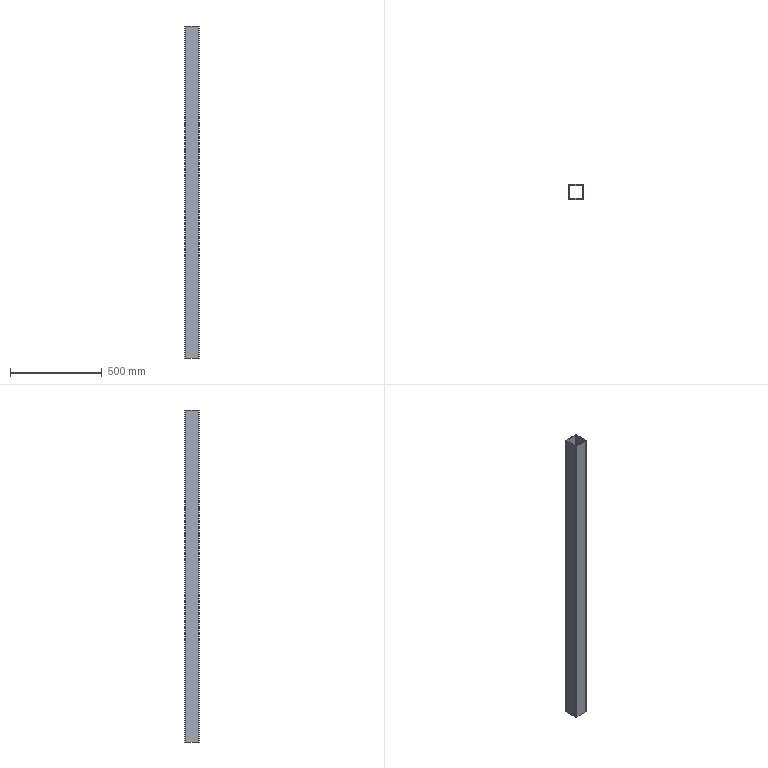Part | SolidWorks | features Extrusion 1 | 1 solid | 18 faces | box 81 x 81 x 1811 mm | volume 2181406 mm3 | plane 10 | cylinder 8 | commonest cylinder face diameters 4 x4 12 x4
STEP:
#1=CARTESIAN_POINT('',(-34.5,40.5,905.5));
#2=VERTEX_POINT('',#1);
#3=CARTESIAN_POINT('',(-40.5,34.5,905.5));
#4=VERTEX_POINT('',#3);
#5=CARTESIAN_POINT('',(-34.5,34.5,905.5));
#6=DIRECTION('',(0.,0.,1.));
#7=DIRECTION('',(1.,0.,0.));
#8=AXIS2_PLACEMENT_3D('',#5,#6,#7);
#9=CIRCLE('',#8,6.);
#10=EDGE_CURVE('',#2,#4,#9,.T.);
#11=ORIENTED_EDGE('',*,*,#10,.T.);
#12=CARTESIAN_POINT('',(-40.5,-34.5,905.5));
#13=VERTEX_POINT('',#12);
#14=CARTESIAN_POINT('',(-40.5,34.5,905.5));
#15=DIRECTION('',(0.,-1.,0.));
#16=VECTOR('',#15,1000.);
#17=LINE('',#14,#16);
#18=EDGE_CURVE('',#4,#13,#17,.T.);
#19=ORIENTED_EDGE('',*,*,#18,.T.);
#20=CARTESIAN_POINT('',(-34.5,-40.5,905.5));
#21=VERTEX_POINT('',#20);
#22=CARTESIAN_POINT('',(-34.5,-34.5,905.5));
#23=DIRECTION('',(0.,0.,1.));
#24=DIRECTION('',(-1.,0.,0.));
#25=AXIS2_PLACEMENT_3D('',#22,#23,#24);
#26=CIRCLE('',#25,6.);
#27=EDGE_CURVE('',#13,#21,#26,.T.);
#28=ORIENTED_EDGE('',*,*,#27,.T.);
#29=CARTESIAN_POINT('',(34.5,-40.5,905.5));
#30=VERTEX_POINT('',#29);
#31=CARTESIAN_POINT('',(34.5,-40.5,905.5));
#32=DIRECTION('',(1.,0.,0.));
#33=VECTOR('',#32,1000.);
#34=LINE('',#31,#33);
#35=EDGE_CURVE('',#21,#30,#34,.T.);
#36=ORIENTED_EDGE('',*,*,#35,.T.);
#37=CARTESIAN_POINT('',(40.5,-34.5,905.5));
#38=VERTEX_POINT('',#37);
#39=CARTESIAN_POINT('',(34.5,-34.5,905.5));
#40=DIRECTION('',(0.,0.,1.));
#41=DIRECTION('',(1.,0.,0.));
#42=AXIS2_PLACEMENT_3D('',#39,#40,#41);
#43=CIRCLE('',#42,6.);
#44=EDGE_CURVE('',#30,#38,#43,.T.);
#45=ORIENTED_EDGE('',*,*,#44,.T.);
#46=CARTESIAN_POINT('',(40.5,34.5,905.5));
#47=VERTEX_POINT('',#46);
#48=CARTESIAN_POINT('',(40.5,-34.5,905.5));
#49=DIRECTION('',(0.,1.,0.));
#50=VECTOR('',#49,1000.);
#51=LINE('',#48,#50);
#52=EDGE_CURVE('',#38,#47,#51,.T.);
#53=ORIENTED_EDGE('',*,*,#52,.T.);
#54=CARTESIAN_POINT('',(34.5,40.5,905.5));
#55=VERTEX_POINT('',#54);
#56=CARTESIAN_POINT('',(34.5,34.5,905.5));
#57=DIRECTION('',(0.,0.,1.));
#58=DIRECTION('',(-1.,0.,0.));
#59=AXIS2_PLACEMENT_3D('',#56,#57,#58);
#60=CIRCLE('',#59,6.);
#61=EDGE_CURVE('',#47,#55,#60,.T.);
#62=ORIENTED_EDGE('',*,*,#61,.T.);
#63=CARTESIAN_POINT('',(0.,40.5,905.5));
#64=DIRECTION('',(-1.,0.,0.));
#65=VECTOR('',#64,1000.);
#66=LINE('',#63,#65);
#67=EDGE_CURVE('',#55,#2,#66,.T.);
#68=ORIENTED_EDGE('',*,*,#67,.T.);
#69=EDGE_LOOP('',(#11,#19,#28,#36,#45,#53,#62,#68));
#70=FACE_OUTER_BOUND('',#69,.T.);
#71=CARTESIAN_POINT('',(-36.5,34.5,905.5));
#72=VERTEX_POINT('',#71);
#73=CARTESIAN_POINT('',(-36.5,-34.5,905.5));
#74=VERTEX_POINT('',#73);
#75=CARTESIAN_POINT('',(-36.5,34.5,905.5));
#76=DIRECTION('',(0.,-1.,0.));
#77=VECTOR('',#76,1000.);
#78=LINE('',#75,#77);
#79=EDGE_CURVE('',#72,#74,#78,.T.);
#80=ORIENTED_EDGE('',*,*,#79,.F.);
#81=CARTESIAN_POINT('',(-34.5,36.5,905.5));
#82=VERTEX_POINT('',#81);
#83=CARTESIAN_POINT('',(-34.5,34.5,905.5));
#84=DIRECTION('',(0.,0.,1.));
#85=DIRECTION('',(1.,0.,0.));
#86=AXIS2_PLACEMENT_3D('',#83,#84,#85);
#87=CIRCLE('',#86,2.);
#88=EDGE_CURVE('',#82,#72,#87,.T.);
#89=ORIENTED_EDGE('',*,*,#88,.F.);
#90=CARTESIAN_POINT('',(34.5,36.5,905.5));
#91=VERTEX_POINT('',#90);
#92=CARTESIAN_POINT('',(0.,36.5,905.5));
#93=DIRECTION('',(-1.,0.,0.));
#94=VECTOR('',#93,1000.);
#95=LINE('',#92,#94);
#96=EDGE_CURVE('',#91,#82,#95,.T.);
#97=ORIENTED_EDGE('',*,*,#96,.F.);
#98=CARTESIAN_POINT('',(36.5,34.5,905.5));
#99=VERTEX_POINT('',#98);
#100=CARTESIAN_POINT('',(34.5,34.5,905.5));
#101=DIRECTION('',(0.,0.,1.));
#102=DIRECTION('',(-1.,0.,0.));
#103=AXIS2_PLACEMENT_3D('',#100,#101,#102);
#104=CIRCLE('',#103,2.);
#105=EDGE_CURVE('',#99,#91,#104,.T.);
#106=ORIENTED_EDGE('',*,*,#105,.F.);
#107=CARTESIAN_POINT('',(36.5,-34.5,905.5));
#108=VERTEX_POINT('',#107);
#109=CARTESIAN_POINT('',(36.5,-34.5,905.5));
#110=DIRECTION('',(0.,1.,0.));
#111=VECTOR('',#110,1000.);
#112=LINE('',#109,#111);
#113=EDGE_CURVE('',#108,#99,#112,.T.);
#114=ORIENTED_EDGE('',*,*,#113,.F.);
#115=CARTESIAN_POINT('',(34.5,-36.5,905.5));
#116=VERTEX_POINT('',#115);
#117=CARTESIAN_POINT('',(34.5,-34.5,905.5));
#118=DIRECTION('',(0.,0.,1.));
#119=DIRECTION('',(1.,0.,0.));
#120=AXIS2_PLACEMENT_3D('',#117,#118,#119);
#121=CIRCLE('',#120,2.);
#122=EDGE_CURVE('',#116,#108,#121,.T.);
#123=ORIENTED_EDGE('',*,*,#122,.F.);
#124=CARTESIAN_POINT('',(-34.5,-36.5,905.5));
#125=VERTEX_POINT('',#124);
#126=CARTESIAN_POINT('',(34.5,-36.5,905.5));
#127=DIRECTION('',(1.,0.,0.));
#128=VECTOR('',#127,1000.);
#129=LINE('',#126,#128);
#130=EDGE_CURVE('',#125,#116,#129,.T.);
#131=ORIENTED_EDGE('',*,*,#130,.F.);
#132=CARTESIAN_POINT('',(-34.5,-34.5,905.5));
#133=DIRECTION('',(0.,0.,1.));
#134=DIRECTION('',(-1.,0.,0.));
#135=AXIS2_PLACEMENT_3D('',#132,#133,#134);
#136=CIRCLE('',#135,2.);
#137=EDGE_CURVE('',#74,#125,#136,.T.);
#138=ORIENTED_EDGE('',*,*,#137,.F.);
#139=EDGE_LOOP('',(#80,#89,#97,#106,#114,#123,#131,#138));
#140=FACE_BOUND('',#139,.T.);
#141=CARTESIAN_POINT('',(-34.5,34.5,905.5));
#142=DIRECTION('',(0.,0.,1.));
#143=DIRECTION('',(1.,0.,0.));
#144=AXIS2_PLACEMENT_3D('',#141,#142,#143);
#145=PLANE('',#144);
#146=ADVANCED_FACE('',(#70,#140),#145,.T.);
#147=CARTESIAN_POINT('',(-34.5,40.5,-905.5));
#148=VERTEX_POINT('',#147);
#149=CARTESIAN_POINT('',(-40.5,34.5,-905.5));
#150=VERTEX_POINT('',#149);
#151=CARTESIAN_POINT('',(-34.5,34.5,-905.5));
#152=DIRECTION('',(0.,0.,1.));
#153=DIRECTION('',(1.,0.,0.));
#154=AXIS2_PLACEMENT_3D('',#151,#152,#153);
#155=CIRCLE('',#154,6.);
#156=EDGE_CURVE('',#148,#150,#155,.T.);
#157=ORIENTED_EDGE('',*,*,#156,.F.);
#158=CARTESIAN_POINT('',(34.5,40.5,-905.5));
#159=VERTEX_POINT('',#158);
#160=CARTESIAN_POINT('',(0.,40.5,-905.5));
#161=DIRECTION('',(-1.,0.,0.));
#162=VECTOR('',#161,1000.);
#163=LINE('',#160,#162);
#164=EDGE_CURVE('',#159,#148,#163,.T.);
#165=ORIENTED_EDGE('',*,*,#164,.F.);
#166=CARTESIAN_POINT('',(40.5,34.5,-905.5));
#167=VERTEX_POINT('',#166);
#168=CARTESIAN_POINT('',(34.5,34.5,-905.5));
#169=DIRECTION('',(0.,0.,1.));
#170=DIRECTION('',(-1.,0.,0.));
#171=AXIS2_PLACEMENT_3D('',#168,#169,#170);
#172=CIRCLE('',#171,6.);
#173=EDGE_CURVE('',#167,#159,#172,.T.);
#174=ORIENTED_EDGE('',*,*,#173,.F.);
#175=CARTESIAN_POINT('',(40.5,-34.5,-905.5));
#176=VERTEX_POINT('',#175);
#177=CARTESIAN_POINT('',(40.5,34.5,-905.5));
#178=DIRECTION('',(0.,1.,0.));
#179=VECTOR('',#178,1000.);
#180=LINE('',#177,#179);
#181=EDGE_CURVE('',#176,#167,#180,.T.);
#182=ORIENTED_EDGE('',*,*,#181,.F.);
#183=CARTESIAN_POINT('',(34.5,-40.5,-905.5));
#184=VERTEX_POINT('',#183);
#185=CARTESIAN_POINT('',(34.5,-34.5,-905.5));
#186=DIRECTION('',(0.,0.,1.));
#187=DIRECTION('',(1.,0.,0.));
#188=AXIS2_PLACEMENT_3D('',#185,#186,#187);
#189=CIRCLE('',#188,6.);
#190=EDGE_CURVE('',#184,#176,#189,.T.);
#191=ORIENTED_EDGE('',*,*,#190,.F.);
#192=CARTESIAN_POINT('',(-34.5,-40.5,-905.5));
#193=VERTEX_POINT('',#192);
#194=CARTESIAN_POINT('',(34.5,-40.5,-905.5));
#195=DIRECTION('',(1.,0.,0.));
#196=VECTOR('',#195,1000.);
#197=LINE('',#194,#196);
#198=EDGE_CURVE('',#193,#184,#197,.T.);
#199=ORIENTED_EDGE('',*,*,#198,.F.);
#200=CARTESIAN_POINT('',(-40.5,-34.5,-905.5));
#201=VERTEX_POINT('',#200);
#202=CARTESIAN_POINT('',(-34.5,-34.5,-905.5));
#203=DIRECTION('',(0.,0.,1.));
#204=DIRECTION('',(-1.,0.,0.));
#205=AXIS2_PLACEMENT_3D('',#202,#203,#204);
#206=CIRCLE('',#205,6.);
#207=EDGE_CURVE('',#201,#193,#206,.T.);
#208=ORIENTED_EDGE('',*,*,#207,.F.);
#209=CARTESIAN_POINT('',(-40.5,-34.5,-905.5));
#210=DIRECTION('',(0.,-1.,0.));
#211=VECTOR('',#210,1000.);
#212=LINE('',#209,#211);
#213=EDGE_CURVE('',#150,#201,#212,.T.);
#214=ORIENTED_EDGE('',*,*,#213,.F.);
#215=EDGE_LOOP('',(#157,#165,#174,#182,#191,#199,#208,#214));
#216=FACE_OUTER_BOUND('',#215,.T.);
#217=CARTESIAN_POINT('',(-34.5,36.5,-905.5));
#218=VERTEX_POINT('',#217);
#219=CARTESIAN_POINT('',(-36.5,34.5,-905.5));
#220=VERTEX_POINT('',#219);
#221=CARTESIAN_POINT('',(-34.5,34.5,-905.5));
#222=DIRECTION('',(0.,0.,1.));
#223=DIRECTION('',(1.,0.,0.));
#224=AXIS2_PLACEMENT_3D('',#221,#222,#223);
#225=CIRCLE('',#224,2.);
#226=EDGE_CURVE('',#218,#220,#225,.T.);
#227=ORIENTED_EDGE('',*,*,#226,.T.);
#228=CARTESIAN_POINT('',(-36.5,-34.5,-905.5));
#229=VERTEX_POINT('',#228);
#230=CARTESIAN_POINT('',(-36.5,-34.5,-905.5));
#231=DIRECTION('',(0.,-1.,0.));
#232=VECTOR('',#231,1000.);
#233=LINE('',#230,#232);
#234=EDGE_CURVE('',#220,#229,#233,.T.);
#235=ORIENTED_EDGE('',*,*,#234,.T.);
#236=CARTESIAN_POINT('',(-34.5,-36.5,-905.5));
#237=VERTEX_POINT('',#236);
#238=CARTESIAN_POINT('',(-34.5,-34.5,-905.5));
#239=DIRECTION('',(0.,0.,1.));
#240=DIRECTION('',(-1.,0.,0.));
#241=AXIS2_PLACEMENT_3D('',#238,#239,#240);
#242=CIRCLE('',#241,2.);
#243=EDGE_CURVE('',#229,#237,#242,.T.);
#244=ORIENTED_EDGE('',*,*,#243,.T.);
#245=CARTESIAN_POINT('',(34.5,-36.5,-905.5));
#246=VERTEX_POINT('',#245);
#247=CARTESIAN_POINT('',(34.5,-36.5,-905.5));
#248=DIRECTION('',(1.,0.,0.));
#249=VECTOR('',#248,1000.);
#250=LINE('',#247,#249);
#251=EDGE_CURVE('',#237,#246,#250,.T.);
#252=ORIENTED_EDGE('',*,*,#251,.T.);
#253=CARTESIAN_POINT('',(36.5,-34.5,-905.5));
#254=VERTEX_POINT('',#253);
#255=CARTESIAN_POINT('',(34.5,-34.5,-905.5));
#256=DIRECTION('',(0.,0.,1.));
#257=DIRECTION('',(1.,0.,0.));
#258=AXIS2_PLACEMENT_3D('',#255,#256,#257);
#259=CIRCLE('',#258,2.);
#260=EDGE_CURVE('',#246,#254,#259,.T.);
#261=ORIENTED_EDGE('',*,*,#260,.T.);
#262=CARTESIAN_POINT('',(36.5,34.5,-905.5));
#263=VERTEX_POINT('',#262);
#264=CARTESIAN_POINT('',(36.5,34.5,-905.5));
#265=DIRECTION('',(0.,1.,0.));
#266=VECTOR('',#265,1000.);
#267=LINE('',#264,#266);
#268=EDGE_CURVE('',#254,#263,#267,.T.);
#269=ORIENTED_EDGE('',*,*,#268,.T.);
#270=CARTESIAN_POINT('',(34.5,36.5,-905.5));
#271=VERTEX_POINT('',#270);
#272=CARTESIAN_POINT('',(34.5,34.5,-905.5));
#273=DIRECTION('',(0.,0.,1.));
#274=DIRECTION('',(-1.,0.,0.));
#275=AXIS2_PLACEMENT_3D('',#272,#273,#274);
#276=CIRCLE('',#275,2.);
#277=EDGE_CURVE('',#263,#271,#276,.T.);
#278=ORIENTED_EDGE('',*,*,#277,.T.);
#279=CARTESIAN_POINT('',(0.,36.5,-905.5));
#280=DIRECTION('',(-1.,0.,0.));
#281=VECTOR('',#280,1000.);
#282=LINE('',#279,#281);
#283=EDGE_CURVE('',#271,#218,#282,.T.);
#284=ORIENTED_EDGE('',*,*,#283,.T.);
#285=EDGE_LOOP('',(#227,#235,#244,#252,#261,#269,#278,#284));
#286=FACE_BOUND('',#285,.T.);
#287=CARTESIAN_POINT('',(-34.5,34.5,-905.5));
#288=DIRECTION('',(0.,0.,1.));
#289=DIRECTION('',(1.,0.,0.));
#290=AXIS2_PLACEMENT_3D('',#287,#288,#289);
#291=PLANE('',#290);
#292=ADVANCED_FACE('',(#216,#286),#291,.F.);
#293=ORIENTED_EDGE('',*,*,#156,.T.);
#294=CARTESIAN_POINT('',(-40.5,34.5,905.5));
#295=DIRECTION('',(0.,0.,-1.));
#296=VECTOR('',#295,1000.);
#297=LINE('',#294,#296);
#298=EDGE_CURVE('',#4,#150,#297,.T.);
#299=ORIENTED_EDGE('',*,*,#298,.F.);
#300=ORIENTED_EDGE('',*,*,#10,.F.);
#301=CARTESIAN_POINT('',(-34.5,40.5,905.5));
#302=DIRECTION('',(0.,0.,-1.));
#303=VECTOR('',#302,1000.);
#304=LINE('',#301,#303);
#305=EDGE_CURVE('',#2,#148,#304,.T.);
#306=ORIENTED_EDGE('',*,*,#305,.T.);
#307=EDGE_LOOP('',(#293,#299,#300,#306));
#308=FACE_OUTER_BOUND('',#307,.T.);
#309=CARTESIAN_POINT('',(-34.5,34.5,905.5));
#310=DIRECTION('',(0.,0.,-1.));
#311=DIRECTION('',(-1.,0.,0.));
#312=AXIS2_PLACEMENT_3D('',#309,#310,#311);
#313=CYLINDRICAL_SURFACE('',#312,6.);
#314=ADVANCED_FACE('',(#308),#313,.T.);
#315=ORIENTED_EDGE('',*,*,#213,.T.);
#316=CARTESIAN_POINT('',(-40.5,-34.5,905.5));
#317=DIRECTION('',(0.,0.,-1.));
#318=VECTOR('',#317,1000.);
#319=LINE('',#316,#318);
#320=EDGE_CURVE('',#13,#201,#319,.T.);
#321=ORIENTED_EDGE('',*,*,#320,.F.);
#322=ORIENTED_EDGE('',*,*,#18,.F.);
#323=ORIENTED_EDGE('',*,*,#298,.T.);
#324=EDGE_LOOP('',(#315,#321,#322,#323));
#325=FACE_OUTER_BOUND('',#324,.T.);
#326=CARTESIAN_POINT('',(-40.5,-34.5,905.5));
#327=DIRECTION('',(1.,0.,0.));
#328=DIRECTION('',(0.,1.,0.));
#329=AXIS2_PLACEMENT_3D('',#326,#327,#328);
#330=PLANE('',#329);
#331=ADVANCED_FACE('',(#325),#330,.F.);
#332=ORIENTED_EDGE('',*,*,#207,.T.);
#333=CARTESIAN_POINT('',(-34.5,-40.5,905.5));
#334=DIRECTION('',(0.,0.,-1.));
#335=VECTOR('',#334,1000.);
#336=LINE('',#333,#335);
#337=EDGE_CURVE('',#21,#193,#336,.T.);
#338=ORIENTED_EDGE('',*,*,#337,.F.);
#339=ORIENTED_EDGE('',*,*,#27,.F.);
#340=ORIENTED_EDGE('',*,*,#320,.T.);
#341=EDGE_LOOP('',(#332,#338,#339,#340));
#342=FACE_OUTER_BOUND('',#341,.T.);
#343=CARTESIAN_POINT('',(-34.5,-34.5,905.5));
#344=DIRECTION('',(0.,0.,-1.));
#345=DIRECTION('',(-1.,0.,0.));
#346=AXIS2_PLACEMENT_3D('',#343,#344,#345);
#347=CYLINDRICAL_SURFACE('',#346,6.);
#348=ADVANCED_FACE('',(#342),#347,.T.);
#349=ORIENTED_EDGE('',*,*,#198,.T.);
#350=CARTESIAN_POINT('',(34.5,-40.5,905.5));
#351=DIRECTION('',(0.,0.,-1.));
#352=VECTOR('',#351,1000.);
#353=LINE('',#350,#352);
#354=EDGE_CURVE('',#30,#184,#353,.T.);
#355=ORIENTED_EDGE('',*,*,#354,.F.);
#356=ORIENTED_EDGE('',*,*,#35,.F.);
#357=ORIENTED_EDGE('',*,*,#337,.T.);
#358=EDGE_LOOP('',(#349,#355,#356,#357));
#359=FACE_OUTER_BOUND('',#358,.T.);
#360=CARTESIAN_POINT('',(34.5,-40.5,905.5));
#361=DIRECTION('',(0.,1.,0.));
#362=DIRECTION('',(-1.,0.,0.));
#363=AXIS2_PLACEMENT_3D('',#360,#361,#362);
#364=PLANE('',#363);
#365=ADVANCED_FACE('',(#359),#364,.F.);
#366=ORIENTED_EDGE('',*,*,#190,.T.);
#367=CARTESIAN_POINT('',(40.5,-34.5,905.5));
#368=DIRECTION('',(0.,0.,-1.));
#369=VECTOR('',#368,1000.);
#370=LINE('',#367,#369);
#371=EDGE_CURVE('',#38,#176,#370,.T.);
#372=ORIENTED_EDGE('',*,*,#371,.F.);
#373=ORIENTED_EDGE('',*,*,#44,.F.);
#374=ORIENTED_EDGE('',*,*,#354,.T.);
#375=EDGE_LOOP('',(#366,#372,#373,#374));
#376=FACE_OUTER_BOUND('',#375,.T.);
#377=CARTESIAN_POINT('',(34.5,-34.5,905.5));
#378=DIRECTION('',(0.,0.,-1.));
#379=DIRECTION('',(-1.,0.,0.));
#380=AXIS2_PLACEMENT_3D('',#377,#378,#379);
#381=CYLINDRICAL_SURFACE('',#380,6.);
#382=ADVANCED_FACE('',(#376),#381,.T.);
#383=ORIENTED_EDGE('',*,*,#181,.T.);
#384=CARTESIAN_POINT('',(40.5,34.5,905.5));
#385=DIRECTION('',(0.,0.,-1.));
#386=VECTOR('',#385,1000.);
#387=LINE('',#384,#386);
#388=EDGE_CURVE('',#47,#167,#387,.T.);
#389=ORIENTED_EDGE('',*,*,#388,.F.);
#390=ORIENTED_EDGE('',*,*,#52,.F.);
#391=ORIENTED_EDGE('',*,*,#371,.T.);
#392=EDGE_LOOP('',(#383,#389,#390,#391));
#393=FACE_OUTER_BOUND('',#392,.T.);
#394=CARTESIAN_POINT('',(40.5,34.5,905.5));
#395=DIRECTION('',(-1.,0.,0.));
#396=DIRECTION('',(0.,-1.,0.));
#397=AXIS2_PLACEMENT_3D('',#394,#395,#396);
#398=PLANE('',#397);
#399=ADVANCED_FACE('',(#393),#398,.F.);
#400=ORIENTED_EDGE('',*,*,#173,.T.);
#401=CARTESIAN_POINT('',(34.5,40.5,905.5));
#402=DIRECTION('',(0.,0.,-1.));
#403=VECTOR('',#402,1000.);
#404=LINE('',#401,#403);
#405=EDGE_CURVE('',#55,#159,#404,.T.);
#406=ORIENTED_EDGE('',*,*,#405,.F.);
#407=ORIENTED_EDGE('',*,*,#61,.F.);
#408=ORIENTED_EDGE('',*,*,#388,.T.);
#409=EDGE_LOOP('',(#400,#406,#407,#408));
#410=FACE_OUTER_BOUND('',#409,.T.);
#411=CARTESIAN_POINT('',(34.5,34.5,905.5));
#412=DIRECTION('',(0.,0.,-1.));
#413=DIRECTION('',(-1.,0.,0.));
#414=AXIS2_PLACEMENT_3D('',#411,#412,#413);
#415=CYLINDRICAL_SURFACE('',#414,6.);
#416=ADVANCED_FACE('',(#410),#415,.T.);
#417=ORIENTED_EDGE('',*,*,#164,.T.);
#418=ORIENTED_EDGE('',*,*,#305,.F.);
#419=ORIENTED_EDGE('',*,*,#67,.F.);
#420=ORIENTED_EDGE('',*,*,#405,.T.);
#421=EDGE_LOOP('',(#417,#418,#419,#420));
#422=FACE_OUTER_BOUND('',#421,.T.);
#423=CARTESIAN_POINT('',(0.,40.5,905.5));
#424=DIRECTION('',(0.,-1.,0.));
#425=DIRECTION('',(1.,0.,0.));
#426=AXIS2_PLACEMENT_3D('',#423,#424,#425);
#427=PLANE('',#426);
#428=ADVANCED_FACE('',(#422),#427,.F.);
#429=ORIENTED_EDGE('',*,*,#226,.F.);
#430=CARTESIAN_POINT('',(-34.5,36.5,905.5));
#431=DIRECTION('',(0.,0.,-1.));
#432=VECTOR('',#431,1000.);
#433=LINE('',#430,#432);
#434=EDGE_CURVE('',#82,#218,#433,.T.);
#435=ORIENTED_EDGE('',*,*,#434,.F.);
#436=ORIENTED_EDGE('',*,*,#88,.T.);
#437=CARTESIAN_POINT('',(-36.5,34.5,905.5));
#438=DIRECTION('',(0.,0.,-1.));
#439=VECTOR('',#438,1000.);
#440=LINE('',#437,#439);
#441=EDGE_CURVE('',#72,#220,#440,.T.);
#442=ORIENTED_EDGE('',*,*,#441,.T.);
#443=EDGE_LOOP('',(#429,#435,#436,#442));
#444=FACE_OUTER_BOUND('',#443,.T.);
#445=CARTESIAN_POINT('',(-34.5,34.5,905.5));
#446=DIRECTION('',(0.,0.,-1.));
#447=DIRECTION('',(-1.,0.,0.));
#448=AXIS2_PLACEMENT_3D('',#445,#446,#447);
#449=CYLINDRICAL_SURFACE('',#448,2.);
#450=ADVANCED_FACE('',(#444),#449,.F.);
#451=ORIENTED_EDGE('',*,*,#234,.F.);
#452=ORIENTED_EDGE('',*,*,#441,.F.);
#453=ORIENTED_EDGE('',*,*,#79,.T.);
#454=CARTESIAN_POINT('',(-36.5,-34.5,905.5));
#455=DIRECTION('',(0.,0.,-1.));
#456=VECTOR('',#455,1000.);
#457=LINE('',#454,#456);
#458=EDGE_CURVE('',#74,#229,#457,.T.);
#459=ORIENTED_EDGE('',*,*,#458,.T.);
#460=EDGE_LOOP('',(#451,#452,#453,#459));
#461=FACE_OUTER_BOUND('',#460,.T.);
#462=CARTESIAN_POINT('',(-36.5,-34.5,905.5));
#463=DIRECTION('',(1.,0.,0.));
#464=DIRECTION('',(0.,0.,-1.));
#465=AXIS2_PLACEMENT_3D('',#462,#463,#464);
#466=PLANE('',#465);
#467=ADVANCED_FACE('',(#461),#466,.T.);
#468=ORIENTED_EDGE('',*,*,#243,.F.);
#469=ORIENTED_EDGE('',*,*,#458,.F.);
#470=ORIENTED_EDGE('',*,*,#137,.T.);
#471=CARTESIAN_POINT('',(-34.5,-36.5,905.5));
#472=DIRECTION('',(0.,0.,-1.));
#473=VECTOR('',#472,1000.);
#474=LINE('',#471,#473);
#475=EDGE_CURVE('',#125,#237,#474,.T.);
#476=ORIENTED_EDGE('',*,*,#475,.T.);
#477=EDGE_LOOP('',(#468,#469,#470,#476));
#478=FACE_OUTER_BOUND('',#477,.T.);
#479=CARTESIAN_POINT('',(-34.5,-34.5,905.5));
#480=DIRECTION('',(0.,0.,-1.));
#481=DIRECTION('',(-1.,0.,0.));
#482=AXIS2_PLACEMENT_3D('',#479,#480,#481);
#483=CYLINDRICAL_SURFACE('',#482,2.);
#484=ADVANCED_FACE('',(#478),#483,.F.);
#485=ORIENTED_EDGE('',*,*,#251,.F.);
#486=ORIENTED_EDGE('',*,*,#475,.F.);
#487=ORIENTED_EDGE('',*,*,#130,.T.);
#488=CARTESIAN_POINT('',(34.5,-36.5,905.5));
#489=DIRECTION('',(0.,0.,-1.));
#490=VECTOR('',#489,1000.);
#491=LINE('',#488,#490);
#492=EDGE_CURVE('',#116,#246,#491,.T.);
#493=ORIENTED_EDGE('',*,*,#492,.T.);
#494=EDGE_LOOP('',(#485,#486,#487,#493));
#495=FACE_OUTER_BOUND('',#494,.T.);
#496=CARTESIAN_POINT('',(34.5,-36.5,905.5));
#497=DIRECTION('',(0.,1.,0.));
#498=DIRECTION('',(-1.,0.,0.));
#499=AXIS2_PLACEMENT_3D('',#496,#497,#498);
#500=PLANE('',#499);
#501=ADVANCED_FACE('',(#495),#500,.T.);
#502=ORIENTED_EDGE('',*,*,#260,.F.);
#503=ORIENTED_EDGE('',*,*,#492,.F.);
#504=ORIENTED_EDGE('',*,*,#122,.T.);
#505=CARTESIAN_POINT('',(36.5,-34.5,905.5));
#506=DIRECTION('',(0.,0.,-1.));
#507=VECTOR('',#506,1000.);
#508=LINE('',#505,#507);
#509=EDGE_CURVE('',#108,#254,#508,.T.);
#510=ORIENTED_EDGE('',*,*,#509,.T.);
#511=EDGE_LOOP('',(#502,#503,#504,#510));
#512=FACE_OUTER_BOUND('',#511,.T.);
#513=CARTESIAN_POINT('',(34.5,-34.5,905.5));
#514=DIRECTION('',(0.,0.,-1.));
#515=DIRECTION('',(-1.,0.,0.));
#516=AXIS2_PLACEMENT_3D('',#513,#514,#515);
#517=CYLINDRICAL_SURFACE('',#516,2.);
#518=ADVANCED_FACE('',(#512),#517,.F.);
#519=ORIENTED_EDGE('',*,*,#268,.F.);
#520=ORIENTED_EDGE('',*,*,#509,.F.);
#521=ORIENTED_EDGE('',*,*,#113,.T.);
#522=CARTESIAN_POINT('',(36.5,34.5,905.5));
#523=DIRECTION('',(0.,0.,-1.));
#524=VECTOR('',#523,1000.);
#525=LINE('',#522,#524);
#526=EDGE_CURVE('',#99,#263,#525,.T.);
#527=ORIENTED_EDGE('',*,*,#526,.T.);
#528=EDGE_LOOP('',(#519,#520,#521,#527));
#529=FACE_OUTER_BOUND('',#528,.T.);
#530=CARTESIAN_POINT('',(36.5,34.5,905.5));
#531=DIRECTION('',(-1.,0.,0.));
#532=DIRECTION('',(0.,0.,1.));
#533=AXIS2_PLACEMENT_3D('',#530,#531,#532);
#534=PLANE('',#533);
#535=ADVANCED_FACE('',(#529),#534,.T.);
#536=ORIENTED_EDGE('',*,*,#277,.F.);
#537=ORIENTED_EDGE('',*,*,#526,.F.);
#538=ORIENTED_EDGE('',*,*,#105,.T.);
#539=CARTESIAN_POINT('',(34.5,36.5,905.5));
#540=DIRECTION('',(0.,0.,-1.));
#541=VECTOR('',#540,1000.);
#542=LINE('',#539,#541);
#543=EDGE_CURVE('',#91,#271,#542,.T.);
#544=ORIENTED_EDGE('',*,*,#543,.T.);
#545=EDGE_LOOP('',(#536,#537,#538,#544));
#546=FACE_OUTER_BOUND('',#545,.T.);
#547=CARTESIAN_POINT('',(34.5,34.5,905.5));
#548=DIRECTION('',(0.,0.,-1.));
#549=DIRECTION('',(-1.,0.,0.));
#550=AXIS2_PLACEMENT_3D('',#547,#548,#549);
#551=CYLINDRICAL_SURFACE('',#550,2.);
#552=ADVANCED_FACE('',(#546),#551,.F.);
#553=ORIENTED_EDGE('',*,*,#283,.F.);
#554=ORIENTED_EDGE('',*,*,#543,.F.);
#555=ORIENTED_EDGE('',*,*,#96,.T.);
#556=ORIENTED_EDGE('',*,*,#434,.T.);
#557=EDGE_LOOP('',(#553,#554,#555,#556));
#558=FACE_OUTER_BOUND('',#557,.T.);
#559=CARTESIAN_POINT('',(0.,36.5,905.5));
#560=DIRECTION('',(0.,-1.,0.));
#561=DIRECTION('',(1.,0.,0.));
#562=AXIS2_PLACEMENT_3D('',#559,#560,#561);
#563=PLANE('',#562);
#564=ADVANCED_FACE('',(#558),#563,.T.);
#565=CLOSED_SHELL('',(#146,#292,#314,#331,#348,#365,#382,#399,#416,#428,#450,#467,#484,#501,#518,#535,#552,#564));
#566=MANIFOLD_SOLID_BREP('',#565);
#567=CARTESIAN_POINT('',(0.,0.,0.));
#568=DIRECTION('',(0.,0.,1.));
#569=DIRECTION('',(1.,0.,0.));
#570=AXIS2_PLACEMENT_3D('',#567,#568,#569);
#571=(LENGTH_UNIT()NAMED_UNIT(*)SI_UNIT(.MILLI.,.METRE.));
#572=UNCERTAINTY_MEASURE_WITH_UNIT(LENGTH_MEASURE(0.00001),#571,'','');
#573=(NAMED_UNIT(*)PLANE_ANGLE_UNIT()SI_UNIT($,.RADIAN.));
#574=(NAMED_UNIT(*)SI_UNIT($,.STERADIAN.)SOLID_ANGLE_UNIT());
#575=(GEOMETRIC_REPRESENTATION_CONTEXT(3)GLOBAL_UNCERTAINTY_ASSIGNED_CONTEXT((#572))GLOBAL_UNIT_ASSIGNED_CONTEXT((#571,#573,#574))REPRESENTATION_CONTEXT('',''));
#576=ADVANCED_BREP_SHAPE_REPRESENTATION('',(#566,#570),#575);